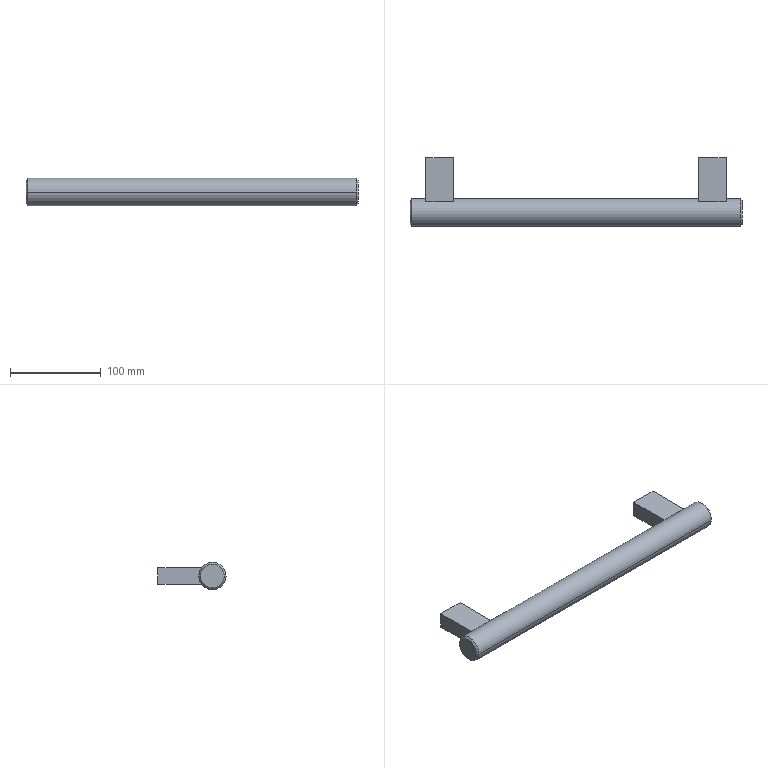Part | NX | features solid 2 | 1 solid | 30 faces | box 365 x 75 x 30 mm | volume 305362 mm3 | plane 12 | cone 12 | cylinder 6 | commonest cylinder face diameters 8 x4 30 x2
STEP:
#1=CARTESIAN_POINT('',(-795.,-1686.,401.));
#2=VERTEX_POINT('',#1);
#3=CARTESIAN_POINT('',(-795.,-1703.,401.));
#4=VERTEX_POINT('',#3);
#5=CARTESIAN_POINT('',(-795.,-1685.,401.));
#6=DIRECTION('',(0.,-1.,0.));
#7=VECTOR('',#6,1000.);
#8=LINE('',#5,#7);
#9=EDGE_CURVE('',#2,#4,#8,.T.);
#10=ORIENTED_EDGE('',*,*,#9,.F.);
#11=CARTESIAN_POINT('',(-791.,-1686.,397.));
#12=VERTEX_POINT('',#11);
#13=CARTESIAN_POINT('',(-795.,-1686.,397.));
#14=DIRECTION('',(0.,1.,0.));
#15=DIRECTION('',(1.,0.,0.));
#16=AXIS2_PLACEMENT_3D('',#13,#14,#15);
#17=CIRCLE('',#16,4.);
#18=EDGE_CURVE('',#2,#12,#17,.T.);
#19=ORIENTED_EDGE('',*,*,#18,.T.);
#20=CARTESIAN_POINT('',(-795.,-1686.,393.));
#21=VERTEX_POINT('',#20);
#22=CARTESIAN_POINT('',(-795.,-1686.,397.));
#23=DIRECTION('',(0.,1.,0.));
#24=DIRECTION('',(1.,0.,0.));
#25=AXIS2_PLACEMENT_3D('',#22,#23,#24);
#26=CIRCLE('',#25,4.);
#27=EDGE_CURVE('',#12,#21,#26,.T.);
#28=ORIENTED_EDGE('',*,*,#27,.T.);
#29=CARTESIAN_POINT('',(-795.,-1703.,393.));
#30=VERTEX_POINT('',#29);
#31=CARTESIAN_POINT('',(-795.,-1685.,393.));
#32=DIRECTION('',(0.,-1.,0.));
#33=VECTOR('',#32,1000.);
#34=LINE('',#31,#33);
#35=EDGE_CURVE('',#30,#21,#34,.F.);
#36=ORIENTED_EDGE('',*,*,#35,.F.);
#37=CARTESIAN_POINT('',(-795.,-1703.,397.));
#38=DIRECTION('',(0.,-1.,0.));
#39=DIRECTION('',(0.,0.,1.));
#40=AXIS2_PLACEMENT_3D('',#37,#38,#39);
#41=CIRCLE('',#40,4.);
#42=EDGE_CURVE('',#30,#4,#41,.T.);
#43=ORIENTED_EDGE('',*,*,#42,.T.);
#44=EDGE_LOOP('',(#10,#19,#28,#36,#43));
#45=FACE_BOUND('',#44,.T.);
#46=CARTESIAN_POINT('',(-795.,-1685.,397.));
#47=DIRECTION('',(0.,-1.,0.));
#48=DIRECTION('',(0.,0.,-1.));
#49=AXIS2_PLACEMENT_3D('',#46,#47,#48);
#50=CYLINDRICAL_SURFACE('',#49,4.);
#51=ADVANCED_FACE('',(#45),#50,.F.);
#52=CARTESIAN_POINT('',(-495.,-1703.,401.));
#53=VERTEX_POINT('',#52);
#54=CARTESIAN_POINT('',(-495.,-1686.,401.));
#55=VERTEX_POINT('',#54);
#56=CARTESIAN_POINT('',(-495.,-1685.,401.));
#57=DIRECTION('',(0.,-1.,0.));
#58=VECTOR('',#57,1000.);
#59=LINE('',#56,#58);
#60=EDGE_CURVE('',#53,#55,#59,.F.);
#61=ORIENTED_EDGE('',*,*,#60,.T.);
#62=CARTESIAN_POINT('',(-491.,-1686.,397.));
#63=VERTEX_POINT('',#62);
#64=CARTESIAN_POINT('',(-495.,-1686.,397.));
#65=DIRECTION('',(0.,1.,0.));
#66=DIRECTION('',(1.,0.,0.));
#67=AXIS2_PLACEMENT_3D('',#64,#65,#66);
#68=CIRCLE('',#67,4.);
#69=EDGE_CURVE('',#55,#63,#68,.T.);
#70=ORIENTED_EDGE('',*,*,#69,.T.);
#71=CARTESIAN_POINT('',(-495.,-1686.,393.));
#72=VERTEX_POINT('',#71);
#73=CARTESIAN_POINT('',(-495.,-1686.,397.));
#74=DIRECTION('',(0.,1.,0.));
#75=DIRECTION('',(1.,0.,0.));
#76=AXIS2_PLACEMENT_3D('',#73,#74,#75);
#77=CIRCLE('',#76,4.);
#78=EDGE_CURVE('',#63,#72,#77,.T.);
#79=ORIENTED_EDGE('',*,*,#78,.T.);
#80=CARTESIAN_POINT('',(-495.,-1703.,393.));
#81=VERTEX_POINT('',#80);
#82=CARTESIAN_POINT('',(-495.,-1685.,393.));
#83=DIRECTION('',(0.,-1.,0.));
#84=VECTOR('',#83,1000.);
#85=LINE('',#82,#84);
#86=EDGE_CURVE('',#72,#81,#85,.T.);
#87=ORIENTED_EDGE('',*,*,#86,.T.);
#88=CARTESIAN_POINT('',(-495.,-1703.,397.));
#89=DIRECTION('',(0.,-1.,0.));
#90=DIRECTION('',(0.,0.,1.));
#91=AXIS2_PLACEMENT_3D('',#88,#89,#90);
#92=CIRCLE('',#91,4.);
#93=EDGE_CURVE('',#81,#53,#92,.T.);
#94=ORIENTED_EDGE('',*,*,#93,.T.);
#95=EDGE_LOOP('',(#61,#70,#79,#87,#94));
#96=FACE_BOUND('',#95,.T.);
#97=CARTESIAN_POINT('',(-495.,-1685.,397.));
#98=DIRECTION('',(0.,-1.,0.));
#99=DIRECTION('',(0.,0.,-1.));
#100=AXIS2_PLACEMENT_3D('',#97,#98,#99);
#101=CYLINDRICAL_SURFACE('',#100,4.);
#102=ADVANCED_FACE('',(#96),#101,.F.);
#103=CARTESIAN_POINT('',(-825.5,-1730.,397.));
#104=VERTEX_POINT('',#103);
#105=CARTESIAN_POINT('',(-810.,-1730.,397.));
#106=VERTEX_POINT('',#105);
#107=CARTESIAN_POINT('',(-827.5,-1730.,397.));
#108=DIRECTION('',(1.,0.,0.));
#109=VECTOR('',#108,1000.);
#110=LINE('',#107,#109);
#111=EDGE_CURVE('',#104,#106,#110,.T.);
#112=ORIENTED_EDGE('',*,*,#111,.F.);
#113=CARTESIAN_POINT('',(-825.5,-1760.,397.));
#114=VERTEX_POINT('',#113);
#115=CARTESIAN_POINT('',(-825.5,-1745.,397.));
#116=DIRECTION('',(-1.,0.,0.));
#117=DIRECTION('',(0.,1.,0.));
#118=AXIS2_PLACEMENT_3D('',#115,#116,#117);
#119=CIRCLE('',#118,15.);
#120=EDGE_CURVE('',#114,#104,#119,.T.);
#121=ORIENTED_EDGE('',*,*,#120,.F.);
#122=CARTESIAN_POINT('',(-464.5,-1760.,397.));
#123=VERTEX_POINT('',#122);
#124=CARTESIAN_POINT('',(-827.5,-1760.,397.));
#125=DIRECTION('',(1.,0.,0.));
#126=VECTOR('',#125,1000.);
#127=LINE('',#124,#126);
#128=EDGE_CURVE('',#123,#114,#127,.F.);
#129=ORIENTED_EDGE('',*,*,#128,.F.);
#130=CARTESIAN_POINT('',(-464.5,-1730.,397.));
#131=VERTEX_POINT('',#130);
#132=CARTESIAN_POINT('',(-464.5,-1745.,397.));
#133=DIRECTION('',(-1.,0.,0.));
#134=DIRECTION('',(0.,1.,0.));
#135=AXIS2_PLACEMENT_3D('',#132,#133,#134);
#136=CIRCLE('',#135,15.);
#137=EDGE_CURVE('',#123,#131,#136,.T.);
#138=ORIENTED_EDGE('',*,*,#137,.T.);
#139=CARTESIAN_POINT('',(-480.,-1730.,397.));
#140=VERTEX_POINT('',#139);
#141=CARTESIAN_POINT('',(-827.5,-1730.,397.));
#142=DIRECTION('',(1.,0.,0.));
#143=VECTOR('',#142,1000.);
#144=LINE('',#141,#143);
#145=EDGE_CURVE('',#140,#131,#144,.T.);
#146=ORIENTED_EDGE('',*,*,#145,.F.);
#147=CARTESIAN_POINT('',(-480.,-1733.,406.));
#148=VERTEX_POINT('',#147);
#149=CARTESIAN_POINT('',(-480.,-1745.,397.));
#150=DIRECTION('',(1.,0.,0.));
#151=DIRECTION('',(0.,0.,1.));
#152=AXIS2_PLACEMENT_3D('',#149,#150,#151);
#153=CIRCLE('',#152,15.);
#154=EDGE_CURVE('',#140,#148,#153,.T.);
#155=ORIENTED_EDGE('',*,*,#154,.T.);
#156=CARTESIAN_POINT('',(-510.,-1733.,406.));
#157=VERTEX_POINT('',#156);
#158=CARTESIAN_POINT('',(-480.,-1733.,406.));
#159=DIRECTION('',(-1.,0.,0.));
#160=VECTOR('',#159,1000.);
#161=LINE('',#158,#160);
#162=EDGE_CURVE('',#148,#157,#161,.T.);
#163=ORIENTED_EDGE('',*,*,#162,.T.);
#164=CARTESIAN_POINT('',(-510.,-1730.,397.));
#165=VERTEX_POINT('',#164);
#166=CARTESIAN_POINT('',(-510.,-1745.,397.));
#167=DIRECTION('',(1.,0.,0.));
#168=DIRECTION('',(0.,0.,1.));
#169=AXIS2_PLACEMENT_3D('',#166,#167,#168);
#170=CIRCLE('',#169,15.);
#171=EDGE_CURVE('',#165,#157,#170,.T.);
#172=ORIENTED_EDGE('',*,*,#171,.F.);
#173=CARTESIAN_POINT('',(-780.,-1730.,397.));
#174=VERTEX_POINT('',#173);
#175=CARTESIAN_POINT('',(-827.5,-1730.,397.));
#176=DIRECTION('',(1.,0.,0.));
#177=VECTOR('',#176,1000.);
#178=LINE('',#175,#177);
#179=EDGE_CURVE('',#174,#165,#178,.T.);
#180=ORIENTED_EDGE('',*,*,#179,.F.);
#181=CARTESIAN_POINT('',(-780.,-1733.,406.));
#182=VERTEX_POINT('',#181);
#183=CARTESIAN_POINT('',(-780.,-1745.,397.));
#184=DIRECTION('',(1.,0.,0.));
#185=DIRECTION('',(0.,0.,1.));
#186=AXIS2_PLACEMENT_3D('',#183,#184,#185);
#187=CIRCLE('',#186,15.);
#188=EDGE_CURVE('',#174,#182,#187,.T.);
#189=ORIENTED_EDGE('',*,*,#188,.T.);
#190=CARTESIAN_POINT('',(-810.,-1733.,406.));
#191=VERTEX_POINT('',#190);
#192=CARTESIAN_POINT('',(-780.,-1733.,406.));
#193=DIRECTION('',(-1.,0.,0.));
#194=VECTOR('',#193,1000.);
#195=LINE('',#192,#194);
#196=EDGE_CURVE('',#182,#191,#195,.T.);
#197=ORIENTED_EDGE('',*,*,#196,.T.);
#198=CARTESIAN_POINT('',(-810.,-1745.,397.));
#199=DIRECTION('',(1.,0.,0.));
#200=DIRECTION('',(0.,0.,1.));
#201=AXIS2_PLACEMENT_3D('',#198,#199,#200);
#202=CIRCLE('',#201,15.);
#203=EDGE_CURVE('',#106,#191,#202,.T.);
#204=ORIENTED_EDGE('',*,*,#203,.F.);
#205=EDGE_LOOP('',(#112,#121,#129,#138,#146,#155,#163,#172,#180,#189,#197,#204));
#206=FACE_BOUND('',#205,.T.);
#207=CARTESIAN_POINT('',(-827.5,-1745.,397.));
#208=DIRECTION('',(1.,0.,0.));
#209=DIRECTION('',(0.,-1.,0.));
#210=AXIS2_PLACEMENT_3D('',#207,#208,#209);
#211=CYLINDRICAL_SURFACE('',#210,15.);
#212=ADVANCED_FACE('',(#206),#211,.T.);
#213=CARTESIAN_POINT('',(-827.5,-1758.,397.));
#214=VERTEX_POINT('',#213);
#215=CARTESIAN_POINT('',(-827.5,-1732.,397.));
#216=VERTEX_POINT('',#215);
#217=CARTESIAN_POINT('',(-827.5,-1745.,397.));
#218=DIRECTION('',(-1.,0.,0.));
#219=DIRECTION('',(0.,1.,0.));
#220=AXIS2_PLACEMENT_3D('',#217,#218,#219);
#221=CIRCLE('',#220,13.);
#222=EDGE_CURVE('',#214,#216,#221,.T.);
#223=ORIENTED_EDGE('',*,*,#222,.T.);
#224=CARTESIAN_POINT('',(-827.5,-1745.,397.));
#225=DIRECTION('',(-1.,0.,0.));
#226=DIRECTION('',(0.,1.,0.));
#227=AXIS2_PLACEMENT_3D('',#224,#225,#226);
#228=CIRCLE('',#227,13.);
#229=EDGE_CURVE('',#216,#214,#228,.T.);
#230=ORIENTED_EDGE('',*,*,#229,.T.);
#231=EDGE_LOOP('',(#223,#230));
#232=FACE_BOUND('',#231,.T.);
#233=CARTESIAN_POINT('',(-827.5,-1745.,397.));
#234=DIRECTION('',(-1.,0.,0.));
#235=DIRECTION('',(0.,1.,0.));
#236=AXIS2_PLACEMENT_3D('',#233,#234,#235);
#237=PLANE('',#236);
#238=ADVANCED_FACE('',(#232),#237,.T.);
#239=CARTESIAN_POINT('',(-462.5,-1732.,397.));
#240=VERTEX_POINT('',#239);
#241=CARTESIAN_POINT('',(-462.5,-1758.,397.));
#242=VERTEX_POINT('',#241);
#243=CARTESIAN_POINT('',(-462.5,-1745.,397.));
#244=DIRECTION('',(-1.,0.,0.));
#245=DIRECTION('',(0.,1.,0.));
#246=AXIS2_PLACEMENT_3D('',#243,#244,#245);
#247=CIRCLE('',#246,13.);
#248=EDGE_CURVE('',#240,#242,#247,.T.);
#249=ORIENTED_EDGE('',*,*,#248,.F.);
#250=CARTESIAN_POINT('',(-462.5,-1745.,397.));
#251=DIRECTION('',(-1.,0.,0.));
#252=DIRECTION('',(0.,1.,0.));
#253=AXIS2_PLACEMENT_3D('',#250,#251,#252);
#254=CIRCLE('',#253,13.);
#255=EDGE_CURVE('',#242,#240,#254,.T.);
#256=ORIENTED_EDGE('',*,*,#255,.F.);
#257=EDGE_LOOP('',(#249,#256));
#258=FACE_BOUND('',#257,.T.);
#259=CARTESIAN_POINT('',(-462.5,-1745.,397.));
#260=DIRECTION('',(-1.,0.,0.));
#261=DIRECTION('',(0.,1.,0.));
#262=AXIS2_PLACEMENT_3D('',#259,#260,#261);
#263=PLANE('',#262);
#264=ADVANCED_FACE('',(#258),#263,.F.);
#265=CARTESIAN_POINT('',(-510.,-1685.,406.));
#266=VERTEX_POINT('',#265);
#267=CARTESIAN_POINT('',(-510.,-1733.,406.));
#268=DIRECTION('',(0.,1.,0.));
#269=VECTOR('',#268,1000.);
#270=LINE('',#267,#269);
#271=EDGE_CURVE('',#157,#266,#270,.T.);
#272=ORIENTED_EDGE('',*,*,#271,.F.);
#273=ORIENTED_EDGE('',*,*,#162,.F.);
#274=CARTESIAN_POINT('',(-480.,-1685.,406.));
#275=VERTEX_POINT('',#274);
#276=CARTESIAN_POINT('',(-480.,-1733.,406.));
#277=DIRECTION('',(0.,1.,0.));
#278=VECTOR('',#277,1000.);
#279=LINE('',#276,#278);
#280=EDGE_CURVE('',#148,#275,#279,.T.);
#281=ORIENTED_EDGE('',*,*,#280,.T.);
#282=CARTESIAN_POINT('',(-480.,-1685.,406.));
#283=DIRECTION('',(-1.,0.,0.));
#284=VECTOR('',#283,1000.);
#285=LINE('',#282,#284);
#286=EDGE_CURVE('',#275,#266,#285,.T.);
#287=ORIENTED_EDGE('',*,*,#286,.T.);
#288=EDGE_LOOP('',(#272,#273,#281,#287));
#289=FACE_BOUND('',#288,.T.);
#290=CARTESIAN_POINT('',(-480.,-1733.,406.));
#291=DIRECTION('',(0.,0.,1.));
#292=DIRECTION('',(0.,-1.,0.));
#293=AXIS2_PLACEMENT_3D('',#290,#291,#292);
#294=PLANE('',#293);
#295=ADVANCED_FACE('',(#289),#294,.T.);
#296=CARTESIAN_POINT('',(-500.,-1685.,397.));
#297=VERTEX_POINT('',#296);
#298=CARTESIAN_POINT('',(-490.,-1685.,397.));
#299=VERTEX_POINT('',#298);
#300=CARTESIAN_POINT('',(-495.,-1685.,397.));
#301=DIRECTION('',(0.,-1.,0.));
#302=DIRECTION('',(-1.,0.,0.));
#303=AXIS2_PLACEMENT_3D('',#300,#301,#302);
#304=CIRCLE('',#303,5.);
#305=EDGE_CURVE('',#297,#299,#304,.T.);
#306=ORIENTED_EDGE('',*,*,#305,.T.);
#307=CARTESIAN_POINT('',(-495.,-1685.,397.));
#308=DIRECTION('',(0.,-1.,0.));
#309=DIRECTION('',(-1.,0.,0.));
#310=AXIS2_PLACEMENT_3D('',#307,#308,#309);
#311=CIRCLE('',#310,5.);
#312=EDGE_CURVE('',#299,#297,#311,.T.);
#313=ORIENTED_EDGE('',*,*,#312,.T.);
#314=EDGE_LOOP('',(#306,#313));
#315=FACE_BOUND('',#314,.T.);
#316=CARTESIAN_POINT('',(-510.,-1685.,388.));
#317=VERTEX_POINT('',#316);
#318=CARTESIAN_POINT('',(-510.,-1685.,406.));
#319=DIRECTION('',(0.,0.,-1.));
#320=VECTOR('',#319,1000.);
#321=LINE('',#318,#320);
#322=EDGE_CURVE('',#266,#317,#321,.T.);
#323=ORIENTED_EDGE('',*,*,#322,.F.);
#324=ORIENTED_EDGE('',*,*,#286,.F.);
#325=CARTESIAN_POINT('',(-480.,-1685.,388.));
#326=VERTEX_POINT('',#325);
#327=CARTESIAN_POINT('',(-480.,-1685.,406.));
#328=DIRECTION('',(0.,0.,-1.));
#329=VECTOR('',#328,1000.);
#330=LINE('',#327,#329);
#331=EDGE_CURVE('',#275,#326,#330,.T.);
#332=ORIENTED_EDGE('',*,*,#331,.T.);
#333=CARTESIAN_POINT('',(-480.,-1685.,388.));
#334=DIRECTION('',(-1.,0.,0.));
#335=VECTOR('',#334,1000.);
#336=LINE('',#333,#335);
#337=EDGE_CURVE('',#326,#317,#336,.T.);
#338=ORIENTED_EDGE('',*,*,#337,.T.);
#339=EDGE_LOOP('',(#323,#324,#332,#338));
#340=FACE_BOUND('',#339,.T.);
#341=CARTESIAN_POINT('',(-480.,-1685.,406.));
#342=DIRECTION('',(0.,1.,0.));
#343=DIRECTION('',(0.,0.,-1.));
#344=AXIS2_PLACEMENT_3D('',#341,#342,#343);
#345=PLANE('',#344);
#346=ADVANCED_FACE('',(#315,#340),#345,.T.);
#347=CARTESIAN_POINT('',(-510.,-1733.,388.));
#348=VERTEX_POINT('',#347);
#349=CARTESIAN_POINT('',(-510.,-1685.,388.));
#350=DIRECTION('',(0.,-1.,0.));
#351=VECTOR('',#350,1000.);
#352=LINE('',#349,#351);
#353=EDGE_CURVE('',#317,#348,#352,.T.);
#354=ORIENTED_EDGE('',*,*,#353,.F.);
#355=ORIENTED_EDGE('',*,*,#337,.F.);
#356=CARTESIAN_POINT('',(-480.,-1733.,388.));
#357=VERTEX_POINT('',#356);
#358=CARTESIAN_POINT('',(-480.,-1685.,388.));
#359=DIRECTION('',(0.,-1.,0.));
#360=VECTOR('',#359,1000.);
#361=LINE('',#358,#360);
#362=EDGE_CURVE('',#326,#357,#361,.T.);
#363=ORIENTED_EDGE('',*,*,#362,.T.);
#364=CARTESIAN_POINT('',(-480.,-1733.,388.));
#365=DIRECTION('',(-1.,0.,0.));
#366=VECTOR('',#365,1000.);
#367=LINE('',#364,#366);
#368=EDGE_CURVE('',#357,#348,#367,.T.);
#369=ORIENTED_EDGE('',*,*,#368,.T.);
#370=EDGE_LOOP('',(#354,#355,#363,#369));
#371=FACE_BOUND('',#370,.T.);
#372=CARTESIAN_POINT('',(-480.,-1685.,388.));
#373=DIRECTION('',(0.,0.,-1.));
#374=DIRECTION('',(0.,-1.,0.));
#375=AXIS2_PLACEMENT_3D('',#372,#373,#374);
#376=PLANE('',#375);
#377=ADVANCED_FACE('',(#371),#376,.T.);
#378=CARTESIAN_POINT('',(-480.,-1745.,397.));
#379=DIRECTION('',(1.,0.,0.));
#380=DIRECTION('',(0.,0.,1.));
#381=AXIS2_PLACEMENT_3D('',#378,#379,#380);
#382=CIRCLE('',#381,15.);
#383=EDGE_CURVE('',#357,#140,#382,.T.);
#384=ORIENTED_EDGE('',*,*,#383,.F.);
#385=ORIENTED_EDGE('',*,*,#362,.F.);
#386=ORIENTED_EDGE('',*,*,#331,.F.);
#387=ORIENTED_EDGE('',*,*,#280,.F.);
#388=ORIENTED_EDGE('',*,*,#154,.F.);
#389=EDGE_LOOP('',(#384,#385,#386,#387,#388));
#390=FACE_BOUND('',#389,.T.);
#391=CARTESIAN_POINT('',(-480.,-1745.,397.));
#392=DIRECTION('',(1.,0.,0.));
#393=DIRECTION('',(0.,1.,0.));
#394=AXIS2_PLACEMENT_3D('',#391,#392,#393);
#395=PLANE('',#394);
#396=ADVANCED_FACE('',(#390),#395,.T.);
#397=CARTESIAN_POINT('',(-510.,-1745.,397.));
#398=DIRECTION('',(1.,0.,0.));
#399=DIRECTION('',(0.,0.,1.));
#400=AXIS2_PLACEMENT_3D('',#397,#398,#399);
#401=CIRCLE('',#400,15.);
#402=EDGE_CURVE('',#348,#165,#401,.T.);
#403=ORIENTED_EDGE('',*,*,#402,.T.);
#404=ORIENTED_EDGE('',*,*,#171,.T.);
#405=ORIENTED_EDGE('',*,*,#271,.T.);
#406=ORIENTED_EDGE('',*,*,#322,.T.);
#407=ORIENTED_EDGE('',*,*,#353,.T.);
#408=EDGE_LOOP('',(#403,#404,#405,#406,#407));
#409=FACE_BOUND('',#408,.T.);
#410=CARTESIAN_POINT('',(-510.,-1745.,397.));
#411=DIRECTION('',(1.,0.,0.));
#412=DIRECTION('',(0.,1.,0.));
#413=AXIS2_PLACEMENT_3D('',#410,#411,#412);
#414=PLANE('',#413);
#415=ADVANCED_FACE('',(#409),#414,.F.);
#416=CARTESIAN_POINT('',(-490.,-1685.,397.));
#417=DIRECTION('',(0.7071,0.7071,0.));
#418=VECTOR('',#417,1000.);
#419=LINE('',#416,#418);
#420=EDGE_CURVE('',#299,#63,#419,.F.);
#421=ORIENTED_EDGE('',*,*,#420,.T.);
#422=ORIENTED_EDGE('',*,*,#69,.F.);
#423=CARTESIAN_POINT('',(-499.,-1686.,397.));
#424=VERTEX_POINT('',#423);
#425=CARTESIAN_POINT('',(-495.,-1686.,397.));
#426=DIRECTION('',(0.,1.,0.));
#427=DIRECTION('',(1.,0.,0.));
#428=AXIS2_PLACEMENT_3D('',#425,#426,#427);
#429=CIRCLE('',#428,4.);
#430=EDGE_CURVE('',#424,#55,#429,.T.);
#431=ORIENTED_EDGE('',*,*,#430,.F.);
#432=CARTESIAN_POINT('',(-500.,-1685.,397.));
#433=DIRECTION('',(-0.7071,0.7071,0.));
#434=VECTOR('',#433,1000.);
#435=LINE('',#432,#434);
#436=EDGE_CURVE('',#424,#297,#435,.T.);
#437=ORIENTED_EDGE('',*,*,#436,.T.);
#438=ORIENTED_EDGE('',*,*,#312,.F.);
#439=EDGE_LOOP('',(#421,#422,#431,#437,#438));
#440=FACE_BOUND('',#439,.T.);
#441=CARTESIAN_POINT('',(-495.,-1685.,397.));
#442=DIRECTION('',(0.,1.,0.));
#443=DIRECTION('',(-1.,0.,0.));
#444=AXIS2_PLACEMENT_3D('',#441,#442,#443);
#445=CONICAL_SURFACE('',#444,5.,0.7854);
#446=ADVANCED_FACE('',(#440),#445,.F.);
#447=CARTESIAN_POINT('',(-495.,-1705.309,397.));
#448=VERTEX_POINT('',#447);
#449=CARTESIAN_POINT('',(-495.,-1703.,393.));
#450=DIRECTION('',(0.,0.5,-0.866));
#451=VECTOR('',#450,1000.);
#452=LINE('',#449,#451);
#453=EDGE_CURVE('',#448,#81,#452,.T.);
#454=ORIENTED_EDGE('',*,*,#453,.F.);
#455=CARTESIAN_POINT('',(-495.,-1703.,401.));
#456=DIRECTION('',(0.,0.5,0.866));
#457=VECTOR('',#456,1000.);
#458=LINE('',#455,#457);
#459=EDGE_CURVE('',#53,#448,#458,.F.);
#460=ORIENTED_EDGE('',*,*,#459,.F.);
#461=ORIENTED_EDGE('',*,*,#93,.F.);
#462=EDGE_LOOP('',(#454,#460,#461));
#463=FACE_BOUND('',#462,.T.);
#464=CARTESIAN_POINT('',(-495.,-1703.,397.));
#465=DIRECTION('',(0.,1.,0.));
#466=DIRECTION('',(0.,0.,1.));
#467=AXIS2_PLACEMENT_3D('',#464,#465,#466);
#468=CONICAL_SURFACE('',#467,4.,1.047);
#469=ADVANCED_FACE('',(#463),#468,.F.);
#470=CARTESIAN_POINT('',(-810.,-1685.,406.));
#471=VERTEX_POINT('',#470);
#472=CARTESIAN_POINT('',(-810.,-1733.,406.));
#473=DIRECTION('',(0.,1.,0.));
#474=VECTOR('',#473,1000.);
#475=LINE('',#472,#474);
#476=EDGE_CURVE('',#191,#471,#475,.T.);
#477=ORIENTED_EDGE('',*,*,#476,.F.);
#478=ORIENTED_EDGE('',*,*,#196,.F.);
#479=CARTESIAN_POINT('',(-780.,-1685.,406.));
#480=VERTEX_POINT('',#479);
#481=CARTESIAN_POINT('',(-780.,-1733.,406.));
#482=DIRECTION('',(0.,1.,0.));
#483=VECTOR('',#482,1000.);
#484=LINE('',#481,#483);
#485=EDGE_CURVE('',#182,#480,#484,.T.);
#486=ORIENTED_EDGE('',*,*,#485,.T.);
#487=CARTESIAN_POINT('',(-780.,-1685.,406.));
#488=DIRECTION('',(-1.,0.,0.));
#489=VECTOR('',#488,1000.);
#490=LINE('',#487,#489);
#491=EDGE_CURVE('',#480,#471,#490,.T.);
#492=ORIENTED_EDGE('',*,*,#491,.T.);
#493=EDGE_LOOP('',(#477,#478,#486,#492));
#494=FACE_BOUND('',#493,.T.);
#495=CARTESIAN_POINT('',(-780.,-1733.,406.));
#496=DIRECTION('',(0.,0.,1.));
#497=DIRECTION('',(0.,-1.,0.));
#498=AXIS2_PLACEMENT_3D('',#495,#496,#497);
#499=PLANE('',#498);
#500=ADVANCED_FACE('',(#494),#499,.T.);
#501=CARTESIAN_POINT('',(-800.,-1685.,397.));
#502=VERTEX_POINT('',#501);
#503=CARTESIAN_POINT('',(-790.,-1685.,397.));
#504=VERTEX_POINT('',#503);
#505=CARTESIAN_POINT('',(-795.,-1685.,397.));
#506=DIRECTION('',(0.,-1.,0.));
#507=DIRECTION('',(-1.,0.,0.));
#508=AXIS2_PLACEMENT_3D('',#505,#506,#507);
#509=CIRCLE('',#508,5.);
#510=EDGE_CURVE('',#502,#504,#509,.T.);
#511=ORIENTED_EDGE('',*,*,#510,.T.);
#512=CARTESIAN_POINT('',(-795.,-1685.,397.));
#513=DIRECTION('',(0.,-1.,0.));
#514=DIRECTION('',(-1.,0.,0.));
#515=AXIS2_PLACEMENT_3D('',#512,#513,#514);
#516=CIRCLE('',#515,5.);
#517=EDGE_CURVE('',#504,#502,#516,.T.);
#518=ORIENTED_EDGE('',*,*,#517,.T.);
#519=EDGE_LOOP('',(#511,#518));
#520=FACE_BOUND('',#519,.T.);
#521=CARTESIAN_POINT('',(-810.,-1685.,388.));
#522=VERTEX_POINT('',#521);
#523=CARTESIAN_POINT('',(-810.,-1685.,406.));
#524=DIRECTION('',(0.,0.,-1.));
#525=VECTOR('',#524,1000.);
#526=LINE('',#523,#525);
#527=EDGE_CURVE('',#471,#522,#526,.T.);
#528=ORIENTED_EDGE('',*,*,#527,.F.);
#529=ORIENTED_EDGE('',*,*,#491,.F.);
#530=CARTESIAN_POINT('',(-780.,-1685.,388.));
#531=VERTEX_POINT('',#530);
#532=CARTESIAN_POINT('',(-780.,-1685.,406.));
#533=DIRECTION('',(0.,0.,-1.));
#534=VECTOR('',#533,1000.);
#535=LINE('',#532,#534);
#536=EDGE_CURVE('',#480,#531,#535,.T.);
#537=ORIENTED_EDGE('',*,*,#536,.T.);
#538=CARTESIAN_POINT('',(-780.,-1685.,388.));
#539=DIRECTION('',(-1.,0.,0.));
#540=VECTOR('',#539,1000.);
#541=LINE('',#538,#540);
#542=EDGE_CURVE('',#531,#522,#541,.T.);
#543=ORIENTED_EDGE('',*,*,#542,.T.);
#544=EDGE_LOOP('',(#528,#529,#537,#543));
#545=FACE_BOUND('',#544,.T.);
#546=CARTESIAN_POINT('',(-780.,-1685.,406.));
#547=DIRECTION('',(0.,1.,0.));
#548=DIRECTION('',(0.,0.,-1.));
#549=AXIS2_PLACEMENT_3D('',#546,#547,#548);
#550=PLANE('',#549);
#551=ADVANCED_FACE('',(#520,#545),#550,.T.);
#552=CARTESIAN_POINT('',(-810.,-1733.,388.));
#553=VERTEX_POINT('',#552);
#554=CARTESIAN_POINT('',(-810.,-1685.,388.));
#555=DIRECTION('',(0.,-1.,0.));
#556=VECTOR('',#555,1000.);
#557=LINE('',#554,#556);
#558=EDGE_CURVE('',#522,#553,#557,.T.);
#559=ORIENTED_EDGE('',*,*,#558,.F.);
#560=ORIENTED_EDGE('',*,*,#542,.F.);
#561=CARTESIAN_POINT('',(-780.,-1733.,388.));
#562=VERTEX_POINT('',#561);
#563=CARTESIAN_POINT('',(-780.,-1685.,388.));
#564=DIRECTION('',(0.,-1.,0.));
#565=VECTOR('',#564,1000.);
#566=LINE('',#563,#565);
#567=EDGE_CURVE('',#531,#562,#566,.T.);
#568=ORIENTED_EDGE('',*,*,#567,.T.);
#569=CARTESIAN_POINT('',(-780.,-1733.,388.));
#570=DIRECTION('',(-1.,0.,0.));
#571=VECTOR('',#570,1000.);
#572=LINE('',#569,#571);
#573=EDGE_CURVE('',#562,#553,#572,.T.);
#574=ORIENTED_EDGE('',*,*,#573,.T.);
#575=EDGE_LOOP('',(#559,#560,#568,#574));
#576=FACE_BOUND('',#575,.T.);
#577=CARTESIAN_POINT('',(-780.,-1685.,388.));
#578=DIRECTION('',(0.,0.,-1.));
#579=DIRECTION('',(0.,-1.,0.));
#580=AXIS2_PLACEMENT_3D('',#577,#578,#579);
#581=PLANE('',#580);
#582=ADVANCED_FACE('',(#576),#581,.T.);
#583=CARTESIAN_POINT('',(-780.,-1745.,397.));
#584=DIRECTION('',(1.,0.,0.));
#585=DIRECTION('',(0.,0.,1.));
#586=AXIS2_PLACEMENT_3D('',#583,#584,#585);
#587=CIRCLE('',#586,15.);
#588=EDGE_CURVE('',#562,#174,#587,.T.);
#589=ORIENTED_EDGE('',*,*,#588,.F.);
#590=ORIENTED_EDGE('',*,*,#567,.F.);
#591=ORIENTED_EDGE('',*,*,#536,.F.);
#592=ORIENTED_EDGE('',*,*,#485,.F.);
#593=ORIENTED_EDGE('',*,*,#188,.F.);
#594=EDGE_LOOP('',(#589,#590,#591,#592,#593));
#595=FACE_BOUND('',#594,.T.);
#596=CARTESIAN_POINT('',(-780.,-1745.,397.));
#597=DIRECTION('',(1.,0.,0.));
#598=DIRECTION('',(0.,1.,0.));
#599=AXIS2_PLACEMENT_3D('',#596,#597,#598);
#600=PLANE('',#599);
#601=ADVANCED_FACE('',(#595),#600,.T.);
#602=CARTESIAN_POINT('',(-810.,-1745.,397.));
#603=DIRECTION('',(1.,0.,0.));
#604=DIRECTION('',(0.,0.,1.));
#605=AXIS2_PLACEMENT_3D('',#602,#603,#604);
#606=CIRCLE('',#605,15.);
#607=EDGE_CURVE('',#553,#106,#606,.T.);
#608=ORIENTED_EDGE('',*,*,#607,.T.);
#609=ORIENTED_EDGE('',*,*,#203,.T.);
#610=ORIENTED_EDGE('',*,*,#476,.T.);
#611=ORIENTED_EDGE('',*,*,#527,.T.);
#612=ORIENTED_EDGE('',*,*,#558,.T.);
#613=EDGE_LOOP('',(#608,#609,#610,#611,#612));
#614=FACE_BOUND('',#613,.T.);
#615=CARTESIAN_POINT('',(-810.,-1745.,397.));
#616=DIRECTION('',(1.,0.,0.));
#617=DIRECTION('',(0.,1.,0.));
#618=AXIS2_PLACEMENT_3D('',#615,#616,#617);
#619=PLANE('',#618);
#620=ADVANCED_FACE('',(#614),#619,.F.);
#621=CARTESIAN_POINT('',(-790.,-1685.,397.));
#622=DIRECTION('',(0.7071,0.7071,0.));
#623=VECTOR('',#622,1000.);
#624=LINE('',#621,#623);
#625=EDGE_CURVE('',#504,#12,#624,.F.);
#626=ORIENTED_EDGE('',*,*,#625,.T.);
#627=ORIENTED_EDGE('',*,*,#18,.F.);
#628=CARTESIAN_POINT('',(-799.,-1686.,397.));
#629=VERTEX_POINT('',#628);
#630=CARTESIAN_POINT('',(-795.,-1686.,397.));
#631=DIRECTION('',(0.,1.,0.));
#632=DIRECTION('',(1.,0.,0.));
#633=AXIS2_PLACEMENT_3D('',#630,#631,#632);
#634=CIRCLE('',#633,4.);
#635=EDGE_CURVE('',#629,#2,#634,.T.);
#636=ORIENTED_EDGE('',*,*,#635,.F.);
#637=CARTESIAN_POINT('',(-800.,-1685.,397.));
#638=DIRECTION('',(-0.7071,0.7071,0.));
#639=VECTOR('',#638,1000.);
#640=LINE('',#637,#639);
#641=EDGE_CURVE('',#629,#502,#640,.T.);
#642=ORIENTED_EDGE('',*,*,#641,.T.);
#643=ORIENTED_EDGE('',*,*,#517,.F.);
#644=EDGE_LOOP('',(#626,#627,#636,#642,#643));
#645=FACE_BOUND('',#644,.T.);
#646=CARTESIAN_POINT('',(-795.,-1685.,397.));
#647=DIRECTION('',(0.,1.,0.));
#648=DIRECTION('',(-1.,0.,0.));
#649=AXIS2_PLACEMENT_3D('',#646,#647,#648);
#650=CONICAL_SURFACE('',#649,5.,0.7854);
#651=ADVANCED_FACE('',(#645),#650,.F.);
#652=CARTESIAN_POINT('',(-795.,-1705.309,397.));
#653=VERTEX_POINT('',#652);
#654=CARTESIAN_POINT('',(-795.,-1703.,393.));
#655=DIRECTION('',(0.,0.5,-0.866));
#656=VECTOR('',#655,1000.);
#657=LINE('',#654,#656);
#658=EDGE_CURVE('',#653,#30,#657,.T.);
#659=ORIENTED_EDGE('',*,*,#658,.F.);
#660=CARTESIAN_POINT('',(-795.,-1703.,401.));
#661=DIRECTION('',(0.,0.5,0.866));
#662=VECTOR('',#661,1000.);
#663=LINE('',#660,#662);
#664=EDGE_CURVE('',#4,#653,#663,.F.);
#665=ORIENTED_EDGE('',*,*,#664,.F.);
#666=ORIENTED_EDGE('',*,*,#42,.F.);
#667=EDGE_LOOP('',(#659,#665,#666));
#668=FACE_BOUND('',#667,.T.);
#669=CARTESIAN_POINT('',(-795.,-1703.,397.));
#670=DIRECTION('',(0.,1.,0.));
#671=DIRECTION('',(0.,0.,1.));
#672=AXIS2_PLACEMENT_3D('',#669,#670,#671);
#673=CONICAL_SURFACE('',#672,4.,1.047);
#674=ADVANCED_FACE('',(#668),#673,.F.);
#675=CARTESIAN_POINT('',(-827.5,-1732.,397.));
#676=DIRECTION('',(0.7071,0.7071,0.));
#677=VECTOR('',#676,1000.);
#678=LINE('',#675,#677);
#679=EDGE_CURVE('',#216,#104,#678,.T.);
#680=ORIENTED_EDGE('',*,*,#679,.F.);
#681=ORIENTED_EDGE('',*,*,#222,.F.);
#682=CARTESIAN_POINT('',(-827.5,-1758.,397.));
#683=DIRECTION('',(0.7071,-0.7071,0.));
#684=VECTOR('',#683,1000.);
#685=LINE('',#682,#684);
#686=EDGE_CURVE('',#114,#214,#685,.F.);
#687=ORIENTED_EDGE('',*,*,#686,.F.);
#688=ORIENTED_EDGE('',*,*,#120,.T.);
#689=EDGE_LOOP('',(#680,#681,#687,#688));
#690=FACE_BOUND('',#689,.T.);
#691=CARTESIAN_POINT('',(-827.5,-1745.,397.));
#692=DIRECTION('',(1.,0.,0.));
#693=DIRECTION('',(0.,-1.,0.));
#694=AXIS2_PLACEMENT_3D('',#691,#692,#693);
#695=CONICAL_SURFACE('',#694,13.,0.7854);
#696=ADVANCED_FACE('',(#690),#695,.T.);
#697=CARTESIAN_POINT('',(-464.5,-1760.,397.));
#698=DIRECTION('',(-0.7071,-0.7071,0.));
#699=VECTOR('',#698,1000.);
#700=LINE('',#697,#699);
#701=EDGE_CURVE('',#123,#242,#700,.F.);
#702=ORIENTED_EDGE('',*,*,#701,.T.);
#703=ORIENTED_EDGE('',*,*,#255,.T.);
#704=CARTESIAN_POINT('',(-464.5,-1730.,397.));
#705=DIRECTION('',(-0.7071,0.7071,0.));
#706=VECTOR('',#705,1000.);
#707=LINE('',#704,#706);
#708=EDGE_CURVE('',#240,#131,#707,.T.);
#709=ORIENTED_EDGE('',*,*,#708,.T.);
#710=ORIENTED_EDGE('',*,*,#137,.F.);
#711=EDGE_LOOP('',(#702,#703,#709,#710));
#712=FACE_BOUND('',#711,.T.);
#713=CARTESIAN_POINT('',(-464.5,-1745.,397.));
#714=DIRECTION('',(-1.,0.,0.));
#715=DIRECTION('',(0.,1.,0.));
#716=AXIS2_PLACEMENT_3D('',#713,#714,#715);
#717=CONICAL_SURFACE('',#716,15.,0.7854);
#718=ADVANCED_FACE('',(#712),#717,.T.);
#719=ORIENTED_EDGE('',*,*,#248,.T.);
#720=ORIENTED_EDGE('',*,*,#701,.F.);
#721=CARTESIAN_POINT('',(-464.5,-1745.,397.));
#722=DIRECTION('',(-1.,0.,0.));
#723=DIRECTION('',(0.,1.,0.));
#724=AXIS2_PLACEMENT_3D('',#721,#722,#723);
#725=CIRCLE('',#724,15.);
#726=EDGE_CURVE('',#131,#123,#725,.T.);
#727=ORIENTED_EDGE('',*,*,#726,.F.);
#728=ORIENTED_EDGE('',*,*,#708,.F.);
#729=EDGE_LOOP('',(#719,#720,#727,#728));
#730=FACE_BOUND('',#729,.T.);
#731=CARTESIAN_POINT('',(-464.5,-1745.,397.));
#732=DIRECTION('',(-1.,0.,0.));
#733=DIRECTION('',(0.,1.,0.));
#734=AXIS2_PLACEMENT_3D('',#731,#732,#733);
#735=CONICAL_SURFACE('',#734,15.,0.7854);
#736=ADVANCED_FACE('',(#730),#735,.T.);
#737=ORIENTED_EDGE('',*,*,#229,.F.);
#738=ORIENTED_EDGE('',*,*,#679,.T.);
#739=CARTESIAN_POINT('',(-825.5,-1745.,397.));
#740=DIRECTION('',(-1.,0.,0.));
#741=DIRECTION('',(0.,1.,0.));
#742=AXIS2_PLACEMENT_3D('',#739,#740,#741);
#743=CIRCLE('',#742,15.);
#744=EDGE_CURVE('',#104,#114,#743,.T.);
#745=ORIENTED_EDGE('',*,*,#744,.T.);
#746=ORIENTED_EDGE('',*,*,#686,.T.);
#747=EDGE_LOOP('',(#737,#738,#745,#746));
#748=FACE_BOUND('',#747,.T.);
#749=CARTESIAN_POINT('',(-827.5,-1745.,397.));
#750=DIRECTION('',(1.,0.,0.));
#751=DIRECTION('',(0.,-1.,0.));
#752=AXIS2_PLACEMENT_3D('',#749,#750,#751);
#753=CONICAL_SURFACE('',#752,13.,0.7854);
#754=ADVANCED_FACE('',(#748),#753,.T.);
#755=ORIENTED_EDGE('',*,*,#664,.T.);
#756=ORIENTED_EDGE('',*,*,#658,.T.);
#757=CARTESIAN_POINT('',(-795.,-1703.,397.));
#758=DIRECTION('',(0.,-1.,0.));
#759=DIRECTION('',(0.,0.,1.));
#760=AXIS2_PLACEMENT_3D('',#757,#758,#759);
#761=CIRCLE('',#760,4.);
#762=EDGE_CURVE('',#4,#30,#761,.T.);
#763=ORIENTED_EDGE('',*,*,#762,.F.);
#764=EDGE_LOOP('',(#755,#756,#763));
#765=FACE_BOUND('',#764,.T.);
#766=CARTESIAN_POINT('',(-795.,-1703.,397.));
#767=DIRECTION('',(0.,1.,0.));
#768=DIRECTION('',(0.,0.,1.));
#769=AXIS2_PLACEMENT_3D('',#766,#767,#768);
#770=CONICAL_SURFACE('',#769,4.,1.047);
#771=ADVANCED_FACE('',(#765),#770,.F.);
#772=ORIENTED_EDGE('',*,*,#27,.F.);
#773=ORIENTED_EDGE('',*,*,#625,.F.);
#774=ORIENTED_EDGE('',*,*,#510,.F.);
#775=ORIENTED_EDGE('',*,*,#641,.F.);
#776=CARTESIAN_POINT('',(-795.,-1686.,397.));
#777=DIRECTION('',(0.,1.,0.));
#778=DIRECTION('',(1.,0.,0.));
#779=AXIS2_PLACEMENT_3D('',#776,#777,#778);
#780=CIRCLE('',#779,4.);
#781=EDGE_CURVE('',#21,#629,#780,.T.);
#782=ORIENTED_EDGE('',*,*,#781,.F.);
#783=EDGE_LOOP('',(#772,#773,#774,#775,#782));
#784=FACE_BOUND('',#783,.T.);
#785=CARTESIAN_POINT('',(-795.,-1685.,397.));
#786=DIRECTION('',(0.,1.,0.));
#787=DIRECTION('',(-1.,0.,0.));
#788=AXIS2_PLACEMENT_3D('',#785,#786,#787);
#789=CONICAL_SURFACE('',#788,5.,0.7854);
#790=ADVANCED_FACE('',(#784),#789,.F.);
#791=ORIENTED_EDGE('',*,*,#459,.T.);
#792=ORIENTED_EDGE('',*,*,#453,.T.);
#793=CARTESIAN_POINT('',(-495.,-1703.,397.));
#794=DIRECTION('',(0.,-1.,0.));
#795=DIRECTION('',(0.,0.,1.));
#796=AXIS2_PLACEMENT_3D('',#793,#794,#795);
#797=CIRCLE('',#796,4.);
#798=EDGE_CURVE('',#53,#81,#797,.T.);
#799=ORIENTED_EDGE('',*,*,#798,.F.);
#800=EDGE_LOOP('',(#791,#792,#799));
#801=FACE_BOUND('',#800,.T.);
#802=CARTESIAN_POINT('',(-495.,-1703.,397.));
#803=DIRECTION('',(0.,1.,0.));
#804=DIRECTION('',(0.,0.,1.));
#805=AXIS2_PLACEMENT_3D('',#802,#803,#804);
#806=CONICAL_SURFACE('',#805,4.,1.047);
#807=ADVANCED_FACE('',(#801),#806,.F.);
#808=ORIENTED_EDGE('',*,*,#78,.F.);
#809=ORIENTED_EDGE('',*,*,#420,.F.);
#810=ORIENTED_EDGE('',*,*,#305,.F.);
#811=ORIENTED_EDGE('',*,*,#436,.F.);
#812=CARTESIAN_POINT('',(-495.,-1686.,397.));
#813=DIRECTION('',(0.,1.,0.));
#814=DIRECTION('',(1.,0.,0.));
#815=AXIS2_PLACEMENT_3D('',#812,#813,#814);
#816=CIRCLE('',#815,4.);
#817=EDGE_CURVE('',#72,#424,#816,.T.);
#818=ORIENTED_EDGE('',*,*,#817,.F.);
#819=EDGE_LOOP('',(#808,#809,#810,#811,#818));
#820=FACE_BOUND('',#819,.T.);
#821=CARTESIAN_POINT('',(-495.,-1685.,397.));
#822=DIRECTION('',(0.,1.,0.));
#823=DIRECTION('',(-1.,0.,0.));
#824=AXIS2_PLACEMENT_3D('',#821,#822,#823);
#825=CONICAL_SURFACE('',#824,5.,0.7854);
#826=ADVANCED_FACE('',(#820),#825,.F.);
#827=ORIENTED_EDGE('',*,*,#744,.F.);
#828=ORIENTED_EDGE('',*,*,#111,.T.);
#829=ORIENTED_EDGE('',*,*,#607,.F.);
#830=ORIENTED_EDGE('',*,*,#573,.F.);
#831=ORIENTED_EDGE('',*,*,#588,.T.);
#832=ORIENTED_EDGE('',*,*,#179,.T.);
#833=ORIENTED_EDGE('',*,*,#402,.F.);
#834=ORIENTED_EDGE('',*,*,#368,.F.);
#835=ORIENTED_EDGE('',*,*,#383,.T.);
#836=ORIENTED_EDGE('',*,*,#145,.T.);
#837=ORIENTED_EDGE('',*,*,#726,.T.);
#838=ORIENTED_EDGE('',*,*,#128,.T.);
#839=EDGE_LOOP('',(#827,#828,#829,#830,#831,#832,#833,#834,#835,#836,#837,#838));
#840=FACE_BOUND('',#839,.T.);
#841=CARTESIAN_POINT('',(-827.5,-1745.,397.));
#842=DIRECTION('',(1.,0.,0.));
#843=DIRECTION('',(0.,-1.,0.));
#844=AXIS2_PLACEMENT_3D('',#841,#842,#843);
#845=CYLINDRICAL_SURFACE('',#844,15.);
#846=ADVANCED_FACE('',(#840),#845,.T.);
#847=ORIENTED_EDGE('',*,*,#430,.T.);
#848=ORIENTED_EDGE('',*,*,#60,.F.);
#849=ORIENTED_EDGE('',*,*,#798,.T.);
#850=ORIENTED_EDGE('',*,*,#86,.F.);
#851=ORIENTED_EDGE('',*,*,#817,.T.);
#852=EDGE_LOOP('',(#847,#848,#849,#850,#851));
#853=FACE_BOUND('',#852,.T.);
#854=CARTESIAN_POINT('',(-495.,-1685.,397.));
#855=DIRECTION('',(0.,-1.,0.));
#856=DIRECTION('',(0.,0.,-1.));
#857=AXIS2_PLACEMENT_3D('',#854,#855,#856);
#858=CYLINDRICAL_SURFACE('',#857,4.);
#859=ADVANCED_FACE('',(#853),#858,.F.);
#860=ORIENTED_EDGE('',*,*,#635,.T.);
#861=ORIENTED_EDGE('',*,*,#9,.T.);
#862=ORIENTED_EDGE('',*,*,#762,.T.);
#863=ORIENTED_EDGE('',*,*,#35,.T.);
#864=ORIENTED_EDGE('',*,*,#781,.T.);
#865=EDGE_LOOP('',(#860,#861,#862,#863,#864));
#866=FACE_BOUND('',#865,.T.);
#867=CARTESIAN_POINT('',(-795.,-1685.,397.));
#868=DIRECTION('',(0.,-1.,0.));
#869=DIRECTION('',(0.,0.,-1.));
#870=AXIS2_PLACEMENT_3D('',#867,#868,#869);
#871=CYLINDRICAL_SURFACE('',#870,4.);
#872=ADVANCED_FACE('',(#866),#871,.F.);
#873=CLOSED_SHELL('',(#51,#102,#212,#238,#264,#295,#346,#377,#396,#415,#446,#469,#500,#551,#582,#601,#620,#651,#674,#696,#718,#736,#754,#771,#790,#807,#826,#846,#859,#872));
#874=MANIFOLD_SOLID_BREP('',#873);
#875=(LENGTH_UNIT()NAMED_UNIT(*)SI_UNIT(.MILLI.,.METRE.));
#876=UNCERTAINTY_MEASURE_WITH_UNIT(LENGTH_MEASURE(0.00001),#875,'','');
#877=(NAMED_UNIT(*)PLANE_ANGLE_UNIT()SI_UNIT($,.RADIAN.));
#878=(NAMED_UNIT(*)SI_UNIT($,.STERADIAN.)SOLID_ANGLE_UNIT());
#879=(GEOMETRIC_REPRESENTATION_CONTEXT(3)GLOBAL_UNCERTAINTY_ASSIGNED_CONTEXT((#876))GLOBAL_UNIT_ASSIGNED_CONTEXT((#875,#877,#878))REPRESENTATION_CONTEXT('',''));
#880=ADVANCED_BREP_SHAPE_REPRESENTATION('',(#874),#879);